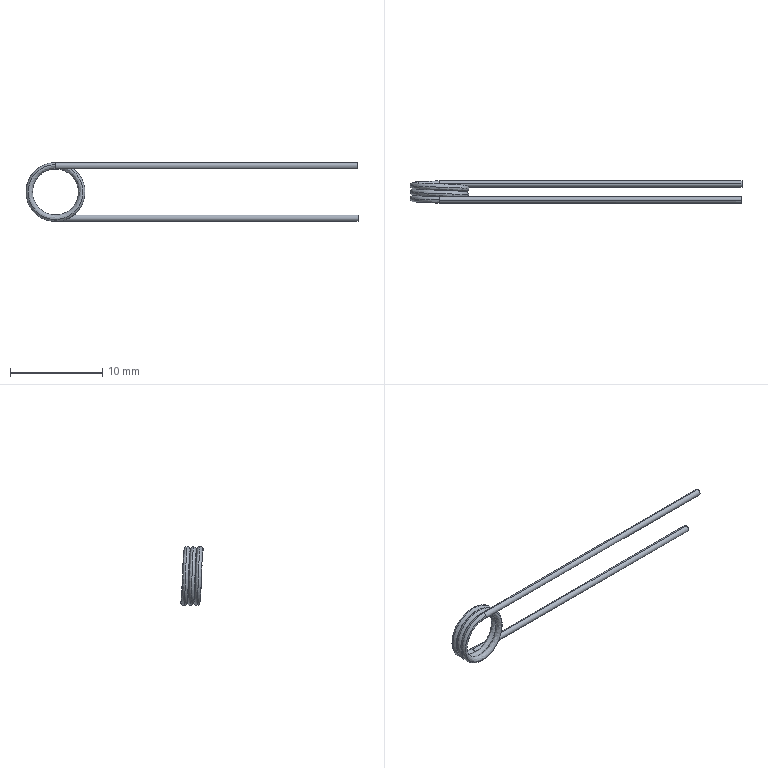Part | SolidWorks | features CompositeCurve 1, Helix 1, MoveFace 1, Sweep 1 | 1 solid | 9 faces | box 36.05 x 2.45 x 6.4 mm | volume 41.978 mm3 | cylinder 4 | spline 3 | plane 2 | commonest cylinder face diameters 0.7 x4
STEP:
#1=CARTESIAN_POINT('',(32.85,1.75,-3.2));
#2=VERTEX_POINT('',#1);
#3=CARTESIAN_POINT('',(32.85,1.75,-2.5));
#4=VERTEX_POINT('',#3);
#5=CARTESIAN_POINT('',(32.85,1.75,-2.85));
#6=DIRECTION('',(1.,0.,0.));
#7=DIRECTION('',(0.,0.00009155,-1.));
#8=AXIS2_PLACEMENT_3D('',#5,#6,#7);
#9=CIRCLE('',#8,0.35);
#10=EDGE_CURVE('',#2,#4,#9,.T.);
#11=ORIENTED_EDGE('',*,*,#10,.F.);
#12=CARTESIAN_POINT('',(-0.000000536,1.75,-3.2));
#13=VERTEX_POINT('',#12);
#14=CARTESIAN_POINT('',(12.85,1.75,-3.2));
#15=DIRECTION('',(-1.,0.,0.));
#16=VECTOR('',#15,1000.);
#17=LINE('',#14,#16);
#18=EDGE_CURVE('',#2,#13,#17,.T.);
#19=ORIENTED_EDGE('',*,*,#18,.T.);
#20=CARTESIAN_POINT('',(-0.006305,2.074,-2.979));
#21=VERTEX_POINT('',#20);
#22=CARTESIAN_POINT('',(0.,1.75,-2.85));
#23=DIRECTION('',(1.,0.,0.));
#24=DIRECTION('',(0.,0.00009155,-1.));
#25=AXIS2_PLACEMENT_3D('',#22,#23,#24);
#26=CIRCLE('',#25,0.35);
#27=EDGE_CURVE('',#13,#21,#26,.T.);
#28=ORIENTED_EDGE('',*,*,#27,.T.);
#29=CARTESIAN_POINT('',(0.,1.75,-2.5));
#30=VERTEX_POINT('',#29);
#31=CARTESIAN_POINT('',(0.,1.75,-2.85));
#32=DIRECTION('',(1.,0.,0.));
#33=DIRECTION('',(0.,0.00009155,-1.));
#34=AXIS2_PLACEMENT_3D('',#31,#32,#33);
#35=CIRCLE('',#34,0.35);
#36=EDGE_CURVE('',#21,#30,#35,.T.);
#37=ORIENTED_EDGE('',*,*,#36,.T.);
#38=CARTESIAN_POINT('',(12.85,1.75,-2.5));
#39=DIRECTION('',(-1.,0.,0.));
#40=VECTOR('',#39,1000.);
#41=LINE('',#38,#40);
#42=EDGE_CURVE('',#4,#30,#41,.T.);
#43=ORIENTED_EDGE('',*,*,#42,.F.);
#44=EDGE_LOOP('',(#11,#19,#28,#37,#43));
#45=FACE_OUTER_BOUND('',#44,.T.);
#46=CARTESIAN_POINT('',(12.85,1.75,-2.85));
#47=DIRECTION('',(-1.,0.,0.));
#48=DIRECTION('',(0.,0.,1.));
#49=AXIS2_PLACEMENT_3D('',#46,#47,#48);
#50=CYLINDRICAL_SURFACE('',#49,0.35);
#51=ADVANCED_FACE('',(#45),#50,.T.);
#52=CARTESIAN_POINT('',(0.006305,0.3239,2.979));
#53=VERTEX_POINT('',#52);
#54=CARTESIAN_POINT('',(0.,0.,3.2));
#55=VERTEX_POINT('',#54);
#56=CARTESIAN_POINT('',(0.006305,0.3239,2.979));
#57=CARTESIAN_POINT('',(0.01048,0.2681,3.104));
#58=CARTESIAN_POINT('',(0.005425,0.1388,3.2));
#59=CARTESIAN_POINT('',(0.,0.,3.2));
#60=B_SPLINE_CURVE_WITH_KNOTS('',3,(#56,#57,#58,#59),.UNSPECIFIED.,.F.,.F.,(4,4),(0.00002721,0.1895),.UNSPECIFIED.);
#61=EDGE_CURVE('',#53,#55,#60,.T.);
#62=ORIENTED_EDGE('',*,*,#61,.T.);
#63=CARTESIAN_POINT('',(32.85,0.,3.2));
#64=VERTEX_POINT('',#63);
#65=CARTESIAN_POINT('',(0.,0.,3.2));
#66=DIRECTION('',(1.,0.,0.));
#67=VECTOR('',#66,1000.);
#68=LINE('',#65,#67);
#69=EDGE_CURVE('',#55,#64,#68,.T.);
#70=ORIENTED_EDGE('',*,*,#69,.T.);
#71=CARTESIAN_POINT('',(32.85,0.,2.5));
#72=VERTEX_POINT('',#71);
#73=CARTESIAN_POINT('',(32.85,0.,2.85));
#74=DIRECTION('',(-1.,0.,0.));
#75=DIRECTION('',(0.,0.,1.));
#76=AXIS2_PLACEMENT_3D('',#73,#74,#75);
#77=CIRCLE('',#76,0.35);
#78=EDGE_CURVE('',#64,#72,#77,.T.);
#79=ORIENTED_EDGE('',*,*,#78,.T.);
#80=CARTESIAN_POINT('',(0.,0.,2.5));
#81=VERTEX_POINT('',#80);
#82=CARTESIAN_POINT('',(0.,0.,2.5));
#83=DIRECTION('',(1.,0.,0.));
#84=VECTOR('',#83,1000.);
#85=LINE('',#82,#84);
#86=EDGE_CURVE('',#81,#72,#85,.T.);
#87=ORIENTED_EDGE('',*,*,#86,.F.);
#88=CARTESIAN_POINT('',(0.,0.,2.85));
#89=DIRECTION('',(-1.,0.,0.));
#90=DIRECTION('',(0.,0.,1.));
#91=AXIS2_PLACEMENT_3D('',#88,#89,#90);
#92=CIRCLE('',#91,0.35);
#93=EDGE_CURVE('',#53,#81,#92,.T.);
#94=ORIENTED_EDGE('',*,*,#93,.F.);
#95=EDGE_LOOP('',(#62,#70,#79,#87,#94));
#96=FACE_OUTER_BOUND('',#95,.T.);
#97=CARTESIAN_POINT('',(0.,0.,2.85));
#98=DIRECTION('',(1.,0.,0.));
#99=DIRECTION('',(0.,0.,-1.));
#100=AXIS2_PLACEMENT_3D('',#97,#98,#99);
#101=CYLINDRICAL_SURFACE('',#100,0.35);
#102=ADVANCED_FACE('',(#96),#101,.T.);
#103=ORIENTED_EDGE('',*,*,#18,.F.);
#104=CARTESIAN_POINT('',(32.85,1.75,-2.85));
#105=DIRECTION('',(1.,0.,0.));
#106=DIRECTION('',(0.,0.00009155,-1.));
#107=AXIS2_PLACEMENT_3D('',#104,#105,#106);
#108=CIRCLE('',#107,0.35);
#109=EDGE_CURVE('',#4,#2,#108,.T.);
#110=ORIENTED_EDGE('',*,*,#109,.F.);
#111=ORIENTED_EDGE('',*,*,#42,.T.);
#112=CARTESIAN_POINT('',(0.006304,1.426,-2.979));
#113=VERTEX_POINT('',#112);
#114=CARTESIAN_POINT('',(0.,1.75,-2.85));
#115=DIRECTION('',(1.,0.,0.));
#116=DIRECTION('',(0.,0.00009155,-1.));
#117=AXIS2_PLACEMENT_3D('',#114,#115,#116);
#118=CIRCLE('',#117,0.35);
#119=EDGE_CURVE('',#30,#113,#118,.T.);
#120=ORIENTED_EDGE('',*,*,#119,.T.);
#121=CARTESIAN_POINT('',(0.,1.75,-2.85));
#122=DIRECTION('',(1.,0.,0.));
#123=DIRECTION('',(0.,0.00009155,-1.));
#124=AXIS2_PLACEMENT_3D('',#121,#122,#123);
#125=CIRCLE('',#124,0.35);
#126=EDGE_CURVE('',#113,#13,#125,.T.);
#127=ORIENTED_EDGE('',*,*,#126,.T.);
#128=EDGE_LOOP('',(#103,#110,#111,#120,#127));
#129=FACE_OUTER_BOUND('',#128,.T.);
#130=CARTESIAN_POINT('',(12.85,1.75,-2.85));
#131=DIRECTION('',(-1.,0.,0.));
#132=DIRECTION('',(0.,0.,1.));
#133=AXIS2_PLACEMENT_3D('',#130,#131,#132);
#134=CYLINDRICAL_SURFACE('',#133,0.35);
#135=ADVANCED_FACE('',(#129),#134,.T.);
#136=ORIENTED_EDGE('',*,*,#36,.F.);
#137=CARTESIAN_POINT('',(0.006305,0.3239,2.979));
#138=CARTESIAN_POINT('',(-0.7712,0.3519,2.981));
#139=CARTESIAN_POINT('',(-1.545,0.381,2.663));
#140=CARTESIAN_POINT('',(-2.649,0.4392,1.566));
#141=CARTESIAN_POINT('',(-2.975,0.4683,0.7939));
#142=CARTESIAN_POINT('',(-2.98,0.5195,-0.5733));
#143=CARTESIAN_POINT('',(-2.806,0.5413,-1.156));
#144=CARTESIAN_POINT('',(-2.162,0.585,-2.13));
#145=CARTESIAN_POINT('',(-1.69,0.6069,-2.521));
#146=CARTESIAN_POINT('',(-0.4324,0.658,-3.048));
#147=CARTESIAN_POINT('',(0.405,0.6871,-3.052));
#148=CARTESIAN_POINT('',(1.67,0.7383,-2.534));
#149=CARTESIAN_POINT('',(2.142,0.7601,-2.15));
#150=CARTESIAN_POINT('',(2.795,0.8037,-1.182));
#151=CARTESIAN_POINT('',(2.976,0.8257,-0.5972));
#152=CARTESIAN_POINT('',(2.981,0.8768,0.7668));
#153=CARTESIAN_POINT('',(2.665,0.9058,1.542));
#154=CARTESIAN_POINT('',(1.702,0.957,2.513));
#155=CARTESIAN_POINT('',(1.167,0.9788,2.801));
#156=CARTESIAN_POINT('',(0.02248,1.022,3.035));
#157=CARTESIAN_POINT('',(-0.587,1.044,2.978));
#158=CARTESIAN_POINT('',(-1.849,1.096,2.461));
#159=CARTESIAN_POINT('',(-2.445,1.125,1.872));
#160=CARTESIAN_POINT('',(-2.973,1.176,0.6109));
#161=CARTESIAN_POINT('',(-3.035,1.198,0.005944));
#162=CARTESIAN_POINT('',(-2.812,1.241,-1.14));
#163=CARTESIAN_POINT('',(-2.526,1.263,-1.682));
#164=CARTESIAN_POINT('',(-1.566,1.314,-2.65));
#165=CARTESIAN_POINT('',(-0.7938,1.343,-2.975));
#166=CARTESIAN_POINT('',(0.5733,1.395,-2.98));
#167=CARTESIAN_POINT('',(1.156,1.416,-2.806));
#168=CARTESIAN_POINT('',(2.13,1.46,-2.162));
#169=CARTESIAN_POINT('',(2.521,1.482,-1.69));
#170=CARTESIAN_POINT('',(3.048,1.533,-0.4324));
#171=CARTESIAN_POINT('',(3.052,1.562,0.405));
#172=CARTESIAN_POINT('',(2.534,1.613,1.67));
#173=CARTESIAN_POINT('',(2.15,1.635,2.142));
#174=CARTESIAN_POINT('',(1.182,1.679,2.795));
#175=CARTESIAN_POINT('',(0.5972,1.701,2.976));
#176=CARTESIAN_POINT('',(-0.7668,1.752,2.981));
#177=CARTESIAN_POINT('',(-1.542,1.781,2.665));
#178=CARTESIAN_POINT('',(-2.513,1.832,1.702));
#179=CARTESIAN_POINT('',(-2.801,1.854,1.167));
#180=CARTESIAN_POINT('',(-3.034,1.897,0.0225));
#181=CARTESIAN_POINT('',(-2.978,1.919,-0.587));
#182=CARTESIAN_POINT('',(-2.46,1.971,-1.85));
#183=CARTESIAN_POINT('',(-1.872,2.,-2.445));
#184=CARTESIAN_POINT('',(-0.7917,2.043,-2.897));
#185=CARTESIAN_POINT('',(-0.4042,2.058,-2.976));
#186=CARTESIAN_POINT('',(-0.006305,2.074,-2.979));
#187=B_SPLINE_CURVE_WITH_KNOTS('',3,(#137,#138,#139,#140,#141,#142,#143,#144,#145,#146,#147,#148,#149,#150,#151,#152,#153,#154,#155,#156,#157,#158,#159,#160,#161,#162,#163,#164,#165,#166,#167,#168,#169,#170,#171,#172,#173,#174,#175,#176,#177,#178,#179,#180,#181,#182,#183,#184,#185,#186),.UNSPECIFIED.,.F.,.F.,(4,2,2,2,2,2,2,2,2,2,2,2,2,2,2,2,2,2,2,2,2,2,2,2,4),(0.,0.04998,0.09999,0.1375,0.175,0.225,0.2625,0.3,0.35,0.3875,0.425,0.475,0.5125,0.55,0.6,0.6375,0.675,0.725,0.7625,0.8,0.85,0.8875,0.925,0.975,1.),.UNSPECIFIED.);
#188=EDGE_CURVE('',#53,#21,#187,.T.);
#189=ORIENTED_EDGE('',*,*,#188,.F.);
#190=ORIENTED_EDGE('',*,*,#93,.T.);
#191=CARTESIAN_POINT('',(-0.006304,-0.3239,2.979));
#192=VERTEX_POINT('',#191);
#193=CARTESIAN_POINT('',(0.,0.,2.85));
#194=DIRECTION('',(-1.,0.,0.));
#195=DIRECTION('',(0.,0.,1.));
#196=AXIS2_PLACEMENT_3D('',#193,#194,#195);
#197=CIRCLE('',#196,0.35);
#198=EDGE_CURVE('',#81,#192,#197,.T.);
#199=ORIENTED_EDGE('',*,*,#198,.T.);
#200=CARTESIAN_POINT('',(0.006304,1.426,-2.979));
#201=CARTESIAN_POINT('',(-0.379,1.413,-2.98));
#202=CARTESIAN_POINT('',(-0.7673,1.398,-2.904));
#203=CARTESIAN_POINT('',(-1.851,1.354,-2.461));
#204=CARTESIAN_POINT('',(-2.445,1.325,-1.871));
#205=CARTESIAN_POINT('',(-2.973,1.274,-0.6122));
#206=CARTESIAN_POINT('',(-3.035,1.252,-0.003211));
#207=CARTESIAN_POINT('',(-2.811,1.209,1.143));
#208=CARTESIAN_POINT('',(-2.527,1.187,1.681));
#209=CARTESIAN_POINT('',(-1.565,1.136,2.652));
#210=CARTESIAN_POINT('',(-0.792,1.107,2.975));
#211=CARTESIAN_POINT('',(0.572,1.056,2.981));
#212=CARTESIAN_POINT('',(1.158,1.034,2.805));
#213=CARTESIAN_POINT('',(2.132,0.99,2.16));
#214=CARTESIAN_POINT('',(2.52,0.9682,1.692));
#215=CARTESIAN_POINT('',(3.049,0.917,0.4308));
#216=CARTESIAN_POINT('',(3.052,0.8879,-0.4067));
#217=CARTESIAN_POINT('',(2.535,0.8368,-1.669));
#218=CARTESIAN_POINT('',(2.148,0.8149,-2.144));
#219=CARTESIAN_POINT('',(1.18,0.7712,-2.796));
#220=CARTESIAN_POINT('',(0.5985,0.7494,-2.976));
#221=CARTESIAN_POINT('',(-0.7686,0.6982,-2.981));
#222=CARTESIAN_POINT('',(-1.544,0.6692,-2.664));
#223=CARTESIAN_POINT('',(-2.512,0.6181,-1.703));
#224=CARTESIAN_POINT('',(-2.802,0.5961,-1.164));
#225=CARTESIAN_POINT('',(-3.035,0.5525,-0.01977));
#226=CARTESIAN_POINT('',(-2.978,0.5307,0.5858));
#227=CARTESIAN_POINT('',(-2.46,0.4795,1.851));
#228=CARTESIAN_POINT('',(-1.87,0.4504,2.445));
#229=CARTESIAN_POINT('',(-0.6122,0.3993,2.973));
#230=CARTESIAN_POINT('',(-0.003226,0.3774,3.035));
#231=CARTESIAN_POINT('',(1.143,0.3337,2.811));
#232=CARTESIAN_POINT('',(1.681,0.3119,2.527));
#233=CARTESIAN_POINT('',(2.652,0.2607,1.565));
#234=CARTESIAN_POINT('',(2.975,0.2317,0.792));
#235=CARTESIAN_POINT('',(2.981,0.1806,-0.572));
#236=CARTESIAN_POINT('',(2.805,0.1586,-1.158));
#237=CARTESIAN_POINT('',(2.16,0.115,-2.132));
#238=CARTESIAN_POINT('',(1.692,0.09317,-2.52));
#239=CARTESIAN_POINT('',(0.4308,0.04196,-3.049));
#240=CARTESIAN_POINT('',(-0.4067,0.01292,-3.052));
#241=CARTESIAN_POINT('',(-1.669,-0.03818,-2.535));
#242=CARTESIAN_POINT('',(-2.144,-0.06013,-2.148));
#243=CARTESIAN_POINT('',(-2.796,-0.1038,-1.18));
#244=CARTESIAN_POINT('',(-2.976,-0.1256,-0.5985));
#245=CARTESIAN_POINT('',(-2.981,-0.1768,0.7687));
#246=CARTESIAN_POINT('',(-2.663,-0.2059,1.544));
#247=CARTESIAN_POINT('',(-1.567,-0.2642,2.65));
#248=CARTESIAN_POINT('',(-0.7966,-0.2932,2.975));
#249=CARTESIAN_POINT('',(-0.006304,-0.3239,2.979));
#250=B_SPLINE_CURVE_WITH_KNOTS('',3,(#200,#201,#202,#203,#204,#205,#206,#207,#208,#209,#210,#211,#212,#213,#214,#215,#216,#217,#218,#219,#220,#221,#222,#223,#224,#225,#226,#227,#228,#229,#230,#231,#232,#233,#234,#235,#236,#237,#238,#239,#240,#241,#242,#243,#244,#245,#246,#247,#248,#249),.UNSPECIFIED.,.F.,.F.,(4,2,2,2,2,2,2,2,2,2,2,2,2,2,2,2,2,2,2,2,2,2,2,2,4),(0.,0.02496,0.07501,0.1125,0.15,0.2,0.2375,0.275,0.325,0.3625,0.4,0.45,0.4875,0.525,0.575,0.6125,0.65,0.7,0.7375,0.775,0.825,0.8625,0.9,0.95,1.),.UNSPECIFIED.);
#251=EDGE_CURVE('',#113,#192,#250,.T.);
#252=ORIENTED_EDGE('',*,*,#251,.F.);
#253=ORIENTED_EDGE('',*,*,#119,.F.);
#254=EDGE_LOOP('',(#136,#189,#190,#199,#252,#253));
#255=FACE_OUTER_BOUND('',#254,.T.);
#256=CARTESIAN_POINT('',(-0.01261,2.073,-2.978));
#257=CARTESIAN_POINT('',(-0.9931,2.036,-2.974));
#258=CARTESIAN_POINT('',(-1.942,2.,-2.452));
#259=CARTESIAN_POINT('',(-3.022,1.927,-0.8338));
#260=CARTESIAN_POINT('',(-3.123,1.89,0.2539));
#261=CARTESIAN_POINT('',(-2.369,1.817,2.048));
#262=CARTESIAN_POINT('',(-1.523,1.781,2.732));
#263=CARTESIAN_POINT('',(0.3864,1.708,3.111));
#264=CARTESIAN_POINT('',(1.43,1.671,2.788));
#265=CARTESIAN_POINT('',(2.798,1.599,1.405));
#266=CARTESIAN_POINT('',(3.107,1.562,0.3615));
#267=CARTESIAN_POINT('',(2.726,1.489,-1.547));
#268=CARTESIAN_POINT('',(2.029,1.453,-2.388));
#269=CARTESIAN_POINT('',(0.2273,1.38,-3.123));
#270=CARTESIAN_POINT('',(-0.8551,1.343,-3.009));
#271=CARTESIAN_POINT('',(-2.473,1.271,-1.927));
#272=CARTESIAN_POINT('',(-2.982,1.234,-0.9604));
#273=CARTESIAN_POINT('',(-2.972,1.161,0.9852));
#274=CARTESIAN_POINT('',(-2.453,1.125,1.942));
#275=CARTESIAN_POINT('',(-0.8335,1.052,3.022));
#276=CARTESIAN_POINT('',(0.2539,1.015,3.123));
#277=CARTESIAN_POINT('',(2.048,0.9425,2.369));
#278=CARTESIAN_POINT('',(2.732,0.9059,1.523));
#279=CARTESIAN_POINT('',(3.111,0.8331,-0.3864));
#280=CARTESIAN_POINT('',(2.788,0.7965,-1.43));
#281=CARTESIAN_POINT('',(1.405,0.7237,-2.798));
#282=CARTESIAN_POINT('',(0.3615,0.6872,-3.107));
#283=CARTESIAN_POINT('',(-1.547,0.6143,-2.726));
#284=CARTESIAN_POINT('',(-2.388,0.5777,-2.029));
#285=CARTESIAN_POINT('',(-3.123,0.505,-0.2273));
#286=CARTESIAN_POINT('',(-3.009,0.4684,0.8554));
#287=CARTESIAN_POINT('',(-1.927,0.3956,2.473));
#288=CARTESIAN_POINT('',(-0.9676,0.3593,2.982));
#289=CARTESIAN_POINT('',(0.01261,0.3226,2.978));
#290=CARTESIAN_POINT('',(-0.0161,2.162,-2.771));
#291=CARTESIAN_POINT('',(-0.9269,2.125,-2.766));
#292=CARTESIAN_POINT('',(-1.811,2.089,-2.279));
#293=CARTESIAN_POINT('',(-2.813,2.016,-0.7712));
#294=CARTESIAN_POINT('',(-2.906,1.979,0.2409));
#295=CARTESIAN_POINT('',(-2.201,1.907,1.909));
#296=CARTESIAN_POINT('',(-1.413,1.87,2.545));
#297=CARTESIAN_POINT('',(0.3644,1.797,2.894));
#298=CARTESIAN_POINT('',(1.334,1.761,2.592));
#299=CARTESIAN_POINT('',(2.606,1.688,1.303));
#300=CARTESIAN_POINT('',(2.892,1.651,0.3318));
#301=CARTESIAN_POINT('',(2.535,1.579,-1.444));
#302=CARTESIAN_POINT('',(1.884,1.542,-2.225));
#303=CARTESIAN_POINT('',(0.2064,1.469,-2.907));
#304=CARTESIAN_POINT('',(-0.8001,1.433,-2.799));
#305=CARTESIAN_POINT('',(-2.304,1.36,-1.789));
#306=CARTESIAN_POINT('',(-2.777,1.323,-0.8894));
#307=CARTESIAN_POINT('',(-2.764,1.25,0.9216));
#308=CARTESIAN_POINT('',(-2.279,1.214,1.81));
#309=CARTESIAN_POINT('',(-0.771,1.141,2.814));
#310=CARTESIAN_POINT('',(0.2409,1.104,2.906));
#311=CARTESIAN_POINT('',(1.909,1.032,2.201));
#312=CARTESIAN_POINT('',(2.545,0.9951,1.413));
#313=CARTESIAN_POINT('',(2.894,0.9223,-0.3644));
#314=CARTESIAN_POINT('',(2.592,0.8857,-1.334));
#315=CARTESIAN_POINT('',(1.303,0.8129,-2.606));
#316=CARTESIAN_POINT('',(0.3318,0.7764,-2.892));
#317=CARTESIAN_POINT('',(-1.444,0.7035,-2.535));
#318=CARTESIAN_POINT('',(-2.225,0.667,-1.884));
#319=CARTESIAN_POINT('',(-2.907,0.5942,-0.2064));
#320=CARTESIAN_POINT('',(-2.798,0.5576,0.8003));
#321=CARTESIAN_POINT('',(-1.789,0.4848,2.304));
#322=CARTESIAN_POINT('',(-0.8958,0.4485,2.776));
#323=CARTESIAN_POINT('',(0.0161,0.4118,2.771));
#324=CARTESIAN_POINT('',(-0.008888,1.977,-2.5));
#325=CARTESIAN_POINT('',(-0.8283,1.941,-2.497));
#326=CARTESIAN_POINT('',(-1.629,1.904,-2.059));
#327=CARTESIAN_POINT('',(-2.536,1.832,-0.7012));
#328=CARTESIAN_POINT('',(-2.622,1.795,0.2114));
#329=CARTESIAN_POINT('',(-1.989,1.722,1.718));
#330=CARTESIAN_POINT('',(-1.28,1.686,2.292));
#331=CARTESIAN_POINT('',(0.3232,1.613,2.612));
#332=CARTESIAN_POINT('',(1.199,1.576,2.341));
#333=CARTESIAN_POINT('',(2.349,1.503,1.18));
#334=CARTESIAN_POINT('',(2.608,1.467,0.3051));
#335=CARTESIAN_POINT('',(2.29,1.394,-1.298));
#336=CARTESIAN_POINT('',(1.704,1.358,-2.003));
#337=CARTESIAN_POINT('',(0.1914,1.285,-2.622));
#338=CARTESIAN_POINT('',(-0.716,1.248,-2.526));
#339=CARTESIAN_POINT('',(-2.075,1.175,-1.618));
#340=CARTESIAN_POINT('',(-2.503,1.139,-0.808));
#341=CARTESIAN_POINT('',(-2.495,1.066,0.8264));
#342=CARTESIAN_POINT('',(-2.06,1.029,1.628));
#343=CARTESIAN_POINT('',(-0.701,0.9565,2.537));
#344=CARTESIAN_POINT('',(0.2114,0.92,2.622));
#345=CARTESIAN_POINT('',(1.718,0.8471,1.989));
#346=CARTESIAN_POINT('',(2.292,0.8107,1.28));
#347=CARTESIAN_POINT('',(2.612,0.7378,-0.3232));
#348=CARTESIAN_POINT('',(2.341,0.7013,-1.199));
#349=CARTESIAN_POINT('',(1.18,0.6284,-2.349));
#350=CARTESIAN_POINT('',(0.3051,0.5919,-2.608));
#351=CARTESIAN_POINT('',(-1.298,0.519,-2.29));
#352=CARTESIAN_POINT('',(-2.003,0.4825,-1.704));
#353=CARTESIAN_POINT('',(-2.622,0.4096,-0.1914));
#354=CARTESIAN_POINT('',(-2.525,0.3732,0.7162));
#355=CARTESIAN_POINT('',(-1.619,0.3003,2.075));
#356=CARTESIAN_POINT('',(-0.8134,0.2639,2.503));
#357=CARTESIAN_POINT('',(0.008889,0.2274,2.5));
#358=CARTESIAN_POINT('',(0.008895,1.522,-2.5));
#359=CARTESIAN_POINT('',(-0.8105,1.486,-2.503));
#360=CARTESIAN_POINT('',(-1.614,1.45,-2.071));
#361=CARTESIAN_POINT('',(-2.532,1.377,-0.7193));
#362=CARTESIAN_POINT('',(-2.623,1.34,0.1927));
#363=CARTESIAN_POINT('',(-2.001,1.267,1.704));
#364=CARTESIAN_POINT('',(-1.296,1.231,2.283));
#365=CARTESIAN_POINT('',(0.3046,1.158,2.614));
#366=CARTESIAN_POINT('',(1.182,1.121,2.35));
#367=CARTESIAN_POINT('',(2.341,1.048,1.197));
#368=CARTESIAN_POINT('',(2.606,1.012,0.3236));
#369=CARTESIAN_POINT('',(2.299,0.9391,-1.282));
#370=CARTESIAN_POINT('',(1.719,0.9026,-1.991));
#371=CARTESIAN_POINT('',(0.2101,0.8297,-2.62));
#372=CARTESIAN_POINT('',(-0.6981,0.7933,-2.531));
#373=CARTESIAN_POINT('',(-2.064,0.7204,-1.633));
#374=CARTESIAN_POINT('',(-2.497,0.6839,-0.8259));
#375=CARTESIAN_POINT('',(-2.501,0.611,0.8087));
#376=CARTESIAN_POINT('',(-2.071,0.5745,1.614));
#377=CARTESIAN_POINT('',(-0.7191,0.5016,2.532));
#378=CARTESIAN_POINT('',(0.1927,0.4651,2.623));
#379=CARTESIAN_POINT('',(1.704,0.3922,2.001));
#380=CARTESIAN_POINT('',(2.283,0.3558,1.296));
#381=CARTESIAN_POINT('',(2.614,0.2829,-0.3046));
#382=CARTESIAN_POINT('',(2.35,0.2464,-1.182));
#383=CARTESIAN_POINT('',(1.197,0.1735,-2.341));
#384=CARTESIAN_POINT('',(0.3236,0.137,-2.606));
#385=CARTESIAN_POINT('',(-1.282,0.0641,-2.299));
#386=CARTESIAN_POINT('',(-1.991,0.02763,-1.719));
#387=CARTESIAN_POINT('',(-2.62,-0.04528,-0.2101));
#388=CARTESIAN_POINT('',(-2.531,-0.08173,0.6983));
#389=CARTESIAN_POINT('',(-1.633,-0.1546,2.064));
#390=CARTESIAN_POINT('',(-0.8313,-0.191,2.497));
#391=CARTESIAN_POINT('',(-0.008894,-0.2275,2.5));
#392=CARTESIAN_POINT('',(0.0161,1.338,-2.771));
#393=CARTESIAN_POINT('',(-0.8947,1.302,-2.777));
#394=CARTESIAN_POINT('',(-1.785,1.265,-2.3));
#395=CARTESIAN_POINT('',(-2.804,1.192,-0.804));
#396=CARTESIAN_POINT('',(-2.908,1.156,0.2071));
#397=CARTESIAN_POINT('',(-2.223,1.083,1.884));
#398=CARTESIAN_POINT('',(-1.443,1.046,2.528));
#399=CARTESIAN_POINT('',(0.3307,0.9736,2.899));
#400=CARTESIAN_POINT('',(1.304,0.937,2.608));
#401=CARTESIAN_POINT('',(2.591,0.8642,1.333));
#402=CARTESIAN_POINT('',(2.888,0.8277,0.3653));
#403=CARTESIAN_POINT('',(2.552,0.7548,-1.415));
#404=CARTESIAN_POINT('',(1.91,0.7183,-2.203));
#405=CARTESIAN_POINT('',(0.2402,0.6455,-2.904));
#406=CARTESIAN_POINT('',(-0.7677,0.6089,-2.808));
#407=CARTESIAN_POINT('',(-2.284,0.5361,-1.816));
#408=CARTESIAN_POINT('',(-2.766,0.4995,-0.9217));
#409=CARTESIAN_POINT('',(-2.775,0.4267,0.8895));
#410=CARTESIAN_POINT('',(-2.3,0.3902,1.784));
#411=CARTESIAN_POINT('',(-0.8038,0.3173,2.805));
#412=CARTESIAN_POINT('',(0.2071,0.2808,2.908));
#413=CARTESIAN_POINT('',(1.884,0.208,2.223));
#414=CARTESIAN_POINT('',(2.528,0.1714,1.443));
#415=CARTESIAN_POINT('',(2.899,0.09857,-0.3307));
#416=CARTESIAN_POINT('',(2.608,0.06204,-1.304));
#417=CARTESIAN_POINT('',(1.333,-0.01079,-2.591));
#418=CARTESIAN_POINT('',(0.3653,-0.0473,-2.888));
#419=CARTESIAN_POINT('',(-1.415,-0.1202,-2.552));
#420=CARTESIAN_POINT('',(-2.203,-0.1567,-1.91));
#421=CARTESIAN_POINT('',(-2.904,-0.2295,-0.2402));
#422=CARTESIAN_POINT('',(-2.807,-0.2661,0.7679));
#423=CARTESIAN_POINT('',(-1.816,-0.3389,2.283));
#424=CARTESIAN_POINT('',(-0.9282,-0.3752,2.766));
#425=CARTESIAN_POINT('',(-0.0161,-0.4119,2.771));
#426=CARTESIAN_POINT('',(0.01261,1.427,-2.978));
#427=CARTESIAN_POINT('',(-0.9679,1.391,-2.982));
#428=CARTESIAN_POINT('',(-1.922,1.354,-2.469));
#429=CARTESIAN_POINT('',(-3.015,1.282,-0.8595));
#430=CARTESIAN_POINT('',(-3.125,1.245,0.2275));
#431=CARTESIAN_POINT('',(-2.386,1.172,2.028));
#432=CARTESIAN_POINT('',(-1.546,1.136,2.72));
#433=CARTESIAN_POINT('',(0.36,1.063,3.114));
#434=CARTESIAN_POINT('',(1.406,1.026,2.8));
#435=CARTESIAN_POINT('',(2.787,0.9536,1.429));
#436=CARTESIAN_POINT('',(3.104,0.917,0.3878));
#437=CARTESIAN_POINT('',(2.739,0.8442,-1.524));
#438=CARTESIAN_POINT('',(2.049,0.8076,-2.37));
#439=CARTESIAN_POINT('',(0.2537,0.7349,-3.121));
#440=CARTESIAN_POINT('',(-0.8297,0.6983,-3.016));
#441=CARTESIAN_POINT('',(-2.457,0.6254,-1.948));
#442=CARTESIAN_POINT('',(-2.974,0.5889,-0.9857));
#443=CARTESIAN_POINT('',(-2.981,0.5161,0.96));
#444=CARTESIAN_POINT('',(-2.469,0.4795,1.921));
#445=CARTESIAN_POINT('',(-0.8592,0.4067,3.015));
#446=CARTESIAN_POINT('',(0.2275,0.3701,3.125));
#447=CARTESIAN_POINT('',(2.028,0.2974,2.386));
#448=CARTESIAN_POINT('',(2.72,0.2608,1.546));
#449=CARTESIAN_POINT('',(3.114,0.1879,-0.36));
#450=CARTESIAN_POINT('',(2.8,0.1514,-1.406));
#451=CARTESIAN_POINT('',(1.429,0.07861,-2.787));
#452=CARTESIAN_POINT('',(0.3878,0.04204,-3.104));
#453=CARTESIAN_POINT('',(-1.524,-0.03081,-2.739));
#454=CARTESIAN_POINT('',(-2.371,-0.06738,-2.049));
#455=CARTESIAN_POINT('',(-3.121,-0.1401,-0.2537));
#456=CARTESIAN_POINT('',(-3.016,-0.1767,0.83));
#457=CARTESIAN_POINT('',(-1.948,-0.2496,2.456));
#458=CARTESIAN_POINT('',(-0.993,-0.2858,2.974));
#459=CARTESIAN_POINT('',(-0.01261,-0.3225,2.978));
#460=B_SPLINE_SURFACE_WITH_KNOTS('',3,3,((#256,#257,#258,#259,#260,#261,#262,#263,#264,#265,#266,#267,#268,#269,#270,#271,#272,#273,#274,#275,#276,#277,#278,#279,#280,#281,#282,#283,#284,#285,#286,#287,#288,#289),(#290,#291,#292,#293,#294,#295,#296,#297,#298,#299,#300,#301,#302,#303,#304,#305,#306,#307,#308,#309,#310,#311,#312,#313,#314,#315,#316,#317,#318,#319,#320,#321,#322,#323),(#324,#325,#326,#327,#328,#329,#330,#331,#332,#333,#334,#335,#336,#337,#338,#339,#340,#341,#342,#343,#344,#345,#346,#347,#348,#349,#350,#351,#352,#353,#354,#355,#356,#357),(#358,#359,#360,#361,#362,#363,#364,#365,#366,#367,#368,#369,#370,#371,#372,#373,#374,#375,#376,#377,#378,#379,#380,#381,#382,#383,#384,#385,#386,#387,#388,#389,#390,#391),(#392,#393,#394,#395,#396,#397,#398,#399,#400,#401,#402,#403,#404,#405,#406,#407,#408,#409,#410,#411,#412,#413,#414,#415,#416,#417,#418,#419,#420,#421,#422,#423,#424,#425),(#426,#427,#428,#429,#430,#431,#432,#433,#434,#435,#436,#437,#438,#439,#440,#441,#442,#443,#444,#445,#446,#447,#448,#449,#450,#451,#452,#453,#454,#455,#456,#457,#458,#459)),.UNSPECIFIED.,.F.,.F.,.F.,(4,2,4),(4,2,2,2,2,2,2,2,2,2,2,2,2,2,2,2,4),(0.1895,0.5,0.8106),(0.,0.0625,0.125,0.1875,0.25,0.3125,0.375,0.4375,0.5,0.5625,0.625,0.6875,0.75,0.8125,0.875,0.9375,1.),.UNSPECIFIED.);
#461=ADVANCED_FACE('',(#255),#460,.F.);
#462=ORIENTED_EDGE('',*,*,#126,.F.);
#463=ORIENTED_EDGE('',*,*,#251,.T.);
#464=CARTESIAN_POINT('',(0.,0.,3.2));
#465=CARTESIAN_POINT('',(-0.005423,-0.1387,3.2));
#466=CARTESIAN_POINT('',(-0.01048,-0.268,3.104));
#467=CARTESIAN_POINT('',(-0.006304,-0.3239,2.979));
#468=B_SPLINE_CURVE_WITH_KNOTS('',3,(#464,#465,#466,#467),.UNSPECIFIED.,.F.,.F.,(4,4),(0.8106,1.),.UNSPECIFIED.);
#469=EDGE_CURVE('',#55,#192,#468,.T.);
#470=ORIENTED_EDGE('',*,*,#469,.F.);
#471=CARTESIAN_POINT('',(-0.000000536,1.75,-3.2));
#472=CARTESIAN_POINT('',(-0.4215,1.735,-3.2));
#473=CARTESIAN_POINT('',(-0.8371,1.721,-3.117));
#474=CARTESIAN_POINT('',(-2.001,1.677,-2.635));
#475=CARTESIAN_POINT('',(-2.635,1.648,-2.));
#476=CARTESIAN_POINT('',(-3.197,1.597,-0.6438));
#477=CARTESIAN_POINT('',(-3.261,1.575,0.01064));
#478=CARTESIAN_POINT('',(-3.015,1.531,1.241));
#479=CARTESIAN_POINT('',(-2.708,1.51,1.817));
#480=CARTESIAN_POINT('',(-1.669,1.458,2.857));
#481=CARTESIAN_POINT('',(-0.8382,1.429,3.2));
#482=CARTESIAN_POINT('',(0.6287,1.378,3.2));
#483=CARTESIAN_POINT('',(1.258,1.356,3.008));
#484=CARTESIAN_POINT('',(2.3,1.313,2.311));
#485=CARTESIAN_POINT('',(2.715,1.291,1.807));
#486=CARTESIAN_POINT('',(3.278,1.239,0.4484));
#487=CARTESIAN_POINT('',(3.277,1.211,-0.4502));
#488=CARTESIAN_POINT('',(2.716,1.159,-1.805));
#489=CARTESIAN_POINT('',(2.298,1.137,-2.313));
#490=CARTESIAN_POINT('',(1.255,1.094,-3.01));
#491=CARTESIAN_POINT('',(0.6301,1.072,-3.2));
#492=CARTESIAN_POINT('',(-0.8402,1.021,-3.2));
#493=CARTESIAN_POINT('',(-1.67,0.9918,-2.855));
#494=CARTESIAN_POINT('',(-2.707,0.9406,-1.818));
#495=CARTESIAN_POINT('',(-3.017,0.9186,-1.238));
#496=CARTESIAN_POINT('',(-3.261,0.875,-0.007701));
#497=CARTESIAN_POINT('',(-3.198,0.8533,0.6424));
#498=CARTESIAN_POINT('',(-2.635,0.8019,2.001));
#499=CARTESIAN_POINT('',(-1.999,0.773,2.636));
#500=CARTESIAN_POINT('',(-0.6438,0.7218,3.197));
#501=CARTESIAN_POINT('',(0.01062,0.6999,3.261));
#502=CARTESIAN_POINT('',(1.241,0.6563,3.015));
#503=CARTESIAN_POINT('',(1.817,0.6345,2.708));
#504=CARTESIAN_POINT('',(2.857,0.5832,1.669));
#505=CARTESIAN_POINT('',(3.2,0.5543,0.8382));
#506=CARTESIAN_POINT('',(3.2,0.5031,-0.6287));
#507=CARTESIAN_POINT('',(3.008,0.4811,-1.258));
#508=CARTESIAN_POINT('',(2.311,0.4375,-2.3));
#509=CARTESIAN_POINT('',(1.807,0.4158,-2.715));
#510=CARTESIAN_POINT('',(0.4484,0.3644,-3.278));
#511=CARTESIAN_POINT('',(-0.4502,0.3355,-3.277));
#512=CARTESIAN_POINT('',(-1.805,0.2843,-2.716));
#513=CARTESIAN_POINT('',(-2.313,0.2624,-2.298));
#514=CARTESIAN_POINT('',(-3.01,0.2188,-1.255));
#515=CARTESIAN_POINT('',(-3.2,0.197,-0.6301));
#516=CARTESIAN_POINT('',(-3.2,0.1457,0.8403));
#517=CARTESIAN_POINT('',(-2.854,0.1167,1.671));
#518=CARTESIAN_POINT('',(-1.671,0.05831,2.854));
#519=CARTESIAN_POINT('',(-0.8425,0.02943,3.2));
#520=CARTESIAN_POINT('',(0.,0.,3.2));
#521=B_SPLINE_CURVE_WITH_KNOTS('',3,(#471,#472,#473,#474,#475,#476,#477,#478,#479,#480,#481,#482,#483,#484,#485,#486,#487,#488,#489,#490,#491,#492,#493,#494,#495,#496,#497,#498,#499,#500,#501,#502,#503,#504,#505,#506,#507,#508,#509,#510,#511,#512,#513,#514,#515,#516,#517,#518,#519,#520),.UNSPECIFIED.,.F.,.F.,(4,2,2,2,2,2,2,2,2,2,2,2,2,2,2,2,2,2,2,2,2,2,2,2,4),(0.,0.02496,0.07501,0.1125,0.15,0.2,0.2375,0.275,0.325,0.3625,0.4,0.45,0.4875,0.525,0.575,0.6125,0.65,0.7,0.7375,0.775,0.825,0.8625,0.9,0.95,1.),.UNSPECIFIED.);
#522=EDGE_CURVE('',#13,#55,#521,.T.);
#523=ORIENTED_EDGE('',*,*,#522,.F.);
#524=EDGE_LOOP('',(#462,#463,#470,#523));
#525=FACE_OUTER_BOUND('',#524,.T.);
#526=CARTESIAN_POINT('',(0.01261,1.427,-2.978));
#527=CARTESIAN_POINT('',(-0.379,1.413,-2.98));
#528=CARTESIAN_POINT('',(-0.7673,1.398,-2.904));
#529=CARTESIAN_POINT('',(-1.851,1.354,-2.461));
#530=CARTESIAN_POINT('',(-2.445,1.325,-1.871));
#531=CARTESIAN_POINT('',(-2.973,1.274,-0.6122));
#532=CARTESIAN_POINT('',(-3.035,1.252,-0.003211));
#533=CARTESIAN_POINT('',(-2.811,1.209,1.143));
#534=CARTESIAN_POINT('',(-2.527,1.187,1.681));
#535=CARTESIAN_POINT('',(-1.565,1.136,2.652));
#536=CARTESIAN_POINT('',(-0.792,1.107,2.975));
#537=CARTESIAN_POINT('',(0.572,1.056,2.981));
#538=CARTESIAN_POINT('',(1.158,1.034,2.805));
#539=CARTESIAN_POINT('',(2.132,0.99,2.16));
#540=CARTESIAN_POINT('',(2.52,0.9682,1.692));
#541=CARTESIAN_POINT('',(3.049,0.917,0.4308));
#542=CARTESIAN_POINT('',(3.052,0.8879,-0.4067));
#543=CARTESIAN_POINT('',(2.535,0.8368,-1.669));
#544=CARTESIAN_POINT('',(2.148,0.8149,-2.144));
#545=CARTESIAN_POINT('',(1.18,0.7712,-2.796));
#546=CARTESIAN_POINT('',(0.5985,0.7494,-2.976));
#547=CARTESIAN_POINT('',(-0.7686,0.6982,-2.981));
#548=CARTESIAN_POINT('',(-1.544,0.6692,-2.664));
#549=CARTESIAN_POINT('',(-2.512,0.6181,-1.703));
#550=CARTESIAN_POINT('',(-2.802,0.5961,-1.164));
#551=CARTESIAN_POINT('',(-3.035,0.5525,-0.01977));
#552=CARTESIAN_POINT('',(-2.978,0.5307,0.5858));
#553=CARTESIAN_POINT('',(-2.46,0.4795,1.851));
#554=CARTESIAN_POINT('',(-1.87,0.4504,2.445));
#555=CARTESIAN_POINT('',(-0.6122,0.3993,2.973));
#556=CARTESIAN_POINT('',(-0.003226,0.3774,3.035));
#557=CARTESIAN_POINT('',(1.143,0.3337,2.811));
#558=CARTESIAN_POINT('',(1.681,0.3119,2.527));
#559=CARTESIAN_POINT('',(2.652,0.2607,1.565));
#560=CARTESIAN_POINT('',(2.975,0.2317,0.792));
#561=CARTESIAN_POINT('',(2.981,0.1806,-0.572));
#562=CARTESIAN_POINT('',(2.805,0.1586,-1.158));
#563=CARTESIAN_POINT('',(2.16,0.115,-2.132));
#564=CARTESIAN_POINT('',(1.692,0.09317,-2.52));
#565=CARTESIAN_POINT('',(0.4308,0.04196,-3.049));
#566=CARTESIAN_POINT('',(-0.4067,0.01292,-3.052));
#567=CARTESIAN_POINT('',(-1.669,-0.03818,-2.535));
#568=CARTESIAN_POINT('',(-2.144,-0.06013,-2.148));
#569=CARTESIAN_POINT('',(-2.796,-0.1038,-1.18));
#570=CARTESIAN_POINT('',(-2.976,-0.1256,-0.5985));
#571=CARTESIAN_POINT('',(-2.981,-0.1768,0.7687));
#572=CARTESIAN_POINT('',(-2.663,-0.2059,1.544));
#573=CARTESIAN_POINT('',(-1.567,-0.2642,2.65));
#574=CARTESIAN_POINT('',(-0.7966,-0.2932,2.975));
#575=CARTESIAN_POINT('',(-0.01261,-0.3225,2.978));
#576=CARTESIAN_POINT('',(0.01048,1.482,-3.104));
#577=CARTESIAN_POINT('',(-0.3981,1.467,-3.106));
#578=CARTESIAN_POINT('',(-0.802,1.453,-3.026));
#579=CARTESIAN_POINT('',(-1.932,1.409,-2.563));
#580=CARTESIAN_POINT('',(-2.55,1.38,-1.948));
#581=CARTESIAN_POINT('',(-3.099,1.329,-0.6352));
#582=CARTESIAN_POINT('',(-3.163,1.307,-0.0004747));
#583=CARTESIAN_POINT('',(-2.929,1.263,1.194));
#584=CARTESIAN_POINT('',(-2.633,1.241,1.754));
#585=CARTESIAN_POINT('',(-1.628,1.19,2.766));
#586=CARTESIAN_POINT('',(-0.8233,1.161,3.102));
#587=CARTESIAN_POINT('',(0.5992,1.11,3.106));
#588=CARTESIAN_POINT('',(1.21,1.088,2.923));
#589=CARTESIAN_POINT('',(2.224,1.044,2.249));
#590=CARTESIAN_POINT('',(2.628,1.023,1.761));
#591=CARTESIAN_POINT('',(3.178,0.9714,0.4459));
#592=CARTESIAN_POINT('',(3.181,0.9425,-0.4263));
#593=CARTESIAN_POINT('',(2.641,0.8913,-1.742));
#594=CARTESIAN_POINT('',(2.237,0.8694,-2.236));
#595=CARTESIAN_POINT('',(1.227,0.8257,-2.915));
#596=CARTESIAN_POINT('',(0.6215,0.804,-3.102));
#597=CARTESIAN_POINT('',(-0.8043,0.7527,-3.107));
#598=CARTESIAN_POINT('',(-1.611,0.7237,-2.775));
#599=CARTESIAN_POINT('',(-2.62,0.6725,-1.773));
#600=CARTESIAN_POINT('',(-2.922,0.6506,-1.211));
#601=CARTESIAN_POINT('',(-3.163,0.607,-0.01804));
#602=CARTESIAN_POINT('',(-3.104,0.5852,0.613));
#603=CARTESIAN_POINT('',(-2.563,0.5339,1.932));
#604=CARTESIAN_POINT('',(-1.948,0.505,2.55));
#605=CARTESIAN_POINT('',(-0.6352,0.4538,3.099));
#606=CARTESIAN_POINT('',(-0.0004918,0.4319,3.163));
#607=CARTESIAN_POINT('',(1.194,0.3882,2.929));
#608=CARTESIAN_POINT('',(1.754,0.3665,2.633));
#609=CARTESIAN_POINT('',(2.766,0.3152,1.628));
#610=CARTESIAN_POINT('',(3.102,0.2862,0.8233));
#611=CARTESIAN_POINT('',(3.106,0.235,-0.5992));
#612=CARTESIAN_POINT('',(2.923,0.2131,-1.21));
#613=CARTESIAN_POINT('',(2.249,0.1695,-2.224));
#614=CARTESIAN_POINT('',(1.761,0.1477,-2.628));
#615=CARTESIAN_POINT('',(0.4459,0.09641,-3.178));
#616=CARTESIAN_POINT('',(-0.4263,0.06746,-3.181));
#617=CARTESIAN_POINT('',(-1.742,0.01629,-2.641));
#618=CARTESIAN_POINT('',(-2.236,-0.005646,-2.237));
#619=CARTESIAN_POINT('',(-2.915,-0.04927,-1.227));
#620=CARTESIAN_POINT('',(-3.102,-0.07105,-0.6215));
#621=CARTESIAN_POINT('',(-3.107,-0.1223,0.8044));
#622=CARTESIAN_POINT('',(-2.774,-0.1514,1.612));
#623=CARTESIAN_POINT('',(-1.631,-0.2097,2.763));
#624=CARTESIAN_POINT('',(-0.8278,-0.2386,3.102));
#625=CARTESIAN_POINT('',(-0.01048,-0.268,3.104));
#626=CARTESIAN_POINT('',(0.005423,1.611,-3.2));
#627=CARTESIAN_POINT('',(-0.416,1.597,-3.201));
#628=CARTESIAN_POINT('',(-0.8318,1.582,-3.118));
#629=CARTESIAN_POINT('',(-1.996,1.538,-2.639));
#630=CARTESIAN_POINT('',(-2.632,1.509,-2.004));
#631=CARTESIAN_POINT('',(-3.196,1.458,-0.6492));
#632=CARTESIAN_POINT('',(-3.261,1.436,0.005106));
#633=CARTESIAN_POINT('',(-3.018,1.393,1.236));
#634=CARTESIAN_POINT('',(-2.711,1.371,1.813));
#635=CARTESIAN_POINT('',(-1.673,1.319,2.854));
#636=CARTESIAN_POINT('',(-0.8436,1.291,3.199));
#637=CARTESIAN_POINT('',(0.6232,1.239,3.201));
#638=CARTESIAN_POINT('',(1.253,1.217,3.011));
#639=CARTESIAN_POINT('',(2.296,1.174,2.315));
#640=CARTESIAN_POINT('',(2.712,1.152,1.811));
#641=CARTESIAN_POINT('',(3.277,1.101,0.4539));
#642=CARTESIAN_POINT('',(3.278,1.072,-0.4446));
#643=CARTESIAN_POINT('',(2.719,1.021,-1.801));
#644=CARTESIAN_POINT('',(2.302,0.9986,-2.309));
#645=CARTESIAN_POINT('',(1.26,0.955,-3.007));
#646=CARTESIAN_POINT('',(0.6356,0.9333,-3.199));
#647=CARTESIAN_POINT('',(-0.8348,0.8819,-3.201));
#648=CARTESIAN_POINT('',(-1.665,0.853,-2.858));
#649=CARTESIAN_POINT('',(-2.704,0.8018,-1.823));
#650=CARTESIAN_POINT('',(-3.014,0.7799,-1.243));
#651=CARTESIAN_POINT('',(-3.261,0.7363,-0.01323));
#652=CARTESIAN_POINT('',(-3.199,0.7145,0.637));
#653=CARTESIAN_POINT('',(-2.638,0.6632,1.996));
#654=CARTESIAN_POINT('',(-2.003,0.6343,2.632));
#655=CARTESIAN_POINT('',(-0.6492,0.583,3.196));
#656=CARTESIAN_POINT('',(0.005088,0.5611,3.261));
#657=CARTESIAN_POINT('',(1.236,0.5175,3.018));
#658=CARTESIAN_POINT('',(1.813,0.4958,2.711));
#659=CARTESIAN_POINT('',(2.854,0.4444,1.673));
#660=CARTESIAN_POINT('',(3.199,0.4155,0.8437));
#661=CARTESIAN_POINT('',(3.201,0.3643,-0.6232));
#662=CARTESIAN_POINT('',(3.011,0.3424,-1.253));
#663=CARTESIAN_POINT('',(2.315,0.2988,-2.296));
#664=CARTESIAN_POINT('',(1.811,0.277,-2.712));
#665=CARTESIAN_POINT('',(0.4539,0.2257,-3.277));
#666=CARTESIAN_POINT('',(-0.4446,0.1968,-3.278));
#667=CARTESIAN_POINT('',(-1.801,0.1455,-2.719));
#668=CARTESIAN_POINT('',(-2.309,0.1236,-2.302));
#669=CARTESIAN_POINT('',(-3.007,0.08004,-1.26));
#670=CARTESIAN_POINT('',(-3.199,0.05826,-0.6356));
#671=CARTESIAN_POINT('',(-3.201,0.006904,0.8348));
#672=CARTESIAN_POINT('',(-2.857,-0.02205,1.666));
#673=CARTESIAN_POINT('',(-1.676,-0.08045,2.852));
#674=CARTESIAN_POINT('',(-0.848,-0.1093,3.199));
#675=CARTESIAN_POINT('',(-0.005424,-0.1388,3.2));
#676=CARTESIAN_POINT('',(-0.000001252,1.75,-3.2));
#677=CARTESIAN_POINT('',(-0.4215,1.735,-3.2));
#678=CARTESIAN_POINT('',(-0.8371,1.721,-3.117));
#679=CARTESIAN_POINT('',(-2.001,1.677,-2.635));
#680=CARTESIAN_POINT('',(-2.635,1.648,-2.));
#681=CARTESIAN_POINT('',(-3.197,1.597,-0.6438));
#682=CARTESIAN_POINT('',(-3.261,1.575,0.01064));
#683=CARTESIAN_POINT('',(-3.015,1.531,1.241));
#684=CARTESIAN_POINT('',(-2.708,1.51,1.817));
#685=CARTESIAN_POINT('',(-1.669,1.458,2.857));
#686=CARTESIAN_POINT('',(-0.8382,1.429,3.2));
#687=CARTESIAN_POINT('',(0.6287,1.378,3.2));
#688=CARTESIAN_POINT('',(1.258,1.356,3.008));
#689=CARTESIAN_POINT('',(2.3,1.313,2.311));
#690=CARTESIAN_POINT('',(2.715,1.291,1.807));
#691=CARTESIAN_POINT('',(3.278,1.239,0.4484));
#692=CARTESIAN_POINT('',(3.277,1.211,-0.4502));
#693=CARTESIAN_POINT('',(2.716,1.159,-1.805));
#694=CARTESIAN_POINT('',(2.298,1.137,-2.313));
#695=CARTESIAN_POINT('',(1.255,1.094,-3.01));
#696=CARTESIAN_POINT('',(0.6301,1.072,-3.2));
#697=CARTESIAN_POINT('',(-0.8402,1.021,-3.2));
#698=CARTESIAN_POINT('',(-1.67,0.9918,-2.855));
#699=CARTESIAN_POINT('',(-2.707,0.9406,-1.818));
#700=CARTESIAN_POINT('',(-3.017,0.9186,-1.238));
#701=CARTESIAN_POINT('',(-3.261,0.875,-0.007701));
#702=CARTESIAN_POINT('',(-3.198,0.8533,0.6424));
#703=CARTESIAN_POINT('',(-2.635,0.8019,2.001));
#704=CARTESIAN_POINT('',(-1.999,0.773,2.636));
#705=CARTESIAN_POINT('',(-0.6438,0.7218,3.197));
#706=CARTESIAN_POINT('',(0.01062,0.6999,3.261));
#707=CARTESIAN_POINT('',(1.241,0.6563,3.015));
#708=CARTESIAN_POINT('',(1.817,0.6345,2.708));
#709=CARTESIAN_POINT('',(2.857,0.5832,1.669));
#710=CARTESIAN_POINT('',(3.2,0.5543,0.8382));
#711=CARTESIAN_POINT('',(3.2,0.5031,-0.6287));
#712=CARTESIAN_POINT('',(3.008,0.4811,-1.258));
#713=CARTESIAN_POINT('',(2.311,0.4375,-2.3));
#714=CARTESIAN_POINT('',(1.807,0.4158,-2.715));
#715=CARTESIAN_POINT('',(0.4484,0.3644,-3.278));
#716=CARTESIAN_POINT('',(-0.4502,0.3355,-3.277));
#717=CARTESIAN_POINT('',(-1.805,0.2843,-2.716));
#718=CARTESIAN_POINT('',(-2.313,0.2624,-2.298));
#719=CARTESIAN_POINT('',(-3.01,0.2188,-1.255));
#720=CARTESIAN_POINT('',(-3.2,0.197,-0.6301));
#721=CARTESIAN_POINT('',(-3.2,0.1457,0.8403));
#722=CARTESIAN_POINT('',(-2.854,0.1167,1.671));
#723=CARTESIAN_POINT('',(-1.671,0.05831,2.854));
#724=CARTESIAN_POINT('',(-0.8425,0.02943,3.2));
#725=CARTESIAN_POINT('',(0.,0.,3.2));
#726=B_SPLINE_SURFACE_WITH_KNOTS('',3,3,((#526,#527,#528,#529,#530,#531,#532,#533,#534,#535,#536,#537,#538,#539,#540,#541,#542,#543,#544,#545,#546,#547,#548,#549,#550,#551,#552,#553,#554,#555,#556,#557,#558,#559,#560,#561,#562,#563,#564,#565,#566,#567,#568,#569,#570,#571,#572,#573,#574,#575),(#576,#577,#578,#579,#580,#581,#582,#583,#584,#585,#586,#587,#588,#589,#590,#591,#592,#593,#594,#595,#596,#597,#598,#599,#600,#601,#602,#603,#604,#605,#606,#607,#608,#609,#610,#611,#612,#613,#614,#615,#616,#617,#618,#619,#620,#621,#622,#623,#624,#625),(#626,#627,#628,#629,#630,#631,#632,#633,#634,#635,#636,#637,#638,#639,#640,#641,#642,#643,#644,#645,#646,#647,#648,#649,#650,#651,#652,#653,#654,#655,#656,#657,#658,#659,#660,#661,#662,#663,#664,#665,#666,#667,#668,#669,#670,#671,#672,#673,#674,#675),(#676,#677,#678,#679,#680,#681,#682,#683,#684,#685,#686,#687,#688,#689,#690,#691,#692,#693,#694,#695,#696,#697,#698,#699,#700,#701,#702,#703,#704,#705,#706,#707,#708,#709,#710,#711,#712,#713,#714,#715,#716,#717,#718,#719,#720,#721,#722,#723,#724,#725)),.UNSPECIFIED.,.F.,.F.,.F.,(4,4),(4,2,2,2,2,2,2,2,2,2,2,2,2,2,2,2,2,2,2,2,2,2,2,2,4),(0.8106,1.),(0.,0.02496,0.07501,0.1125,0.15,0.2,0.2375,0.275,0.325,0.3625,0.4,0.45,0.4875,0.525,0.575,0.6125,0.65,0.7,0.7375,0.775,0.825,0.8625,0.9,0.95,1.),.UNSPECIFIED.);
#727=ADVANCED_FACE('',(#525),#726,.F.);
#728=ORIENTED_EDGE('',*,*,#27,.F.);
#729=ORIENTED_EDGE('',*,*,#522,.T.);
#730=ORIENTED_EDGE('',*,*,#61,.F.);
#731=ORIENTED_EDGE('',*,*,#188,.T.);
#732=EDGE_LOOP('',(#728,#729,#730,#731));
#733=FACE_OUTER_BOUND('',#732,.T.);
#734=CARTESIAN_POINT('',(-0.000001252,1.75,-3.2));
#735=CARTESIAN_POINT('',(-0.4215,1.735,-3.2));
#736=CARTESIAN_POINT('',(-0.8371,1.721,-3.117));
#737=CARTESIAN_POINT('',(-2.001,1.677,-2.635));
#738=CARTESIAN_POINT('',(-2.635,1.648,-2.));
#739=CARTESIAN_POINT('',(-3.197,1.597,-0.6438));
#740=CARTESIAN_POINT('',(-3.261,1.575,0.01064));
#741=CARTESIAN_POINT('',(-3.015,1.531,1.241));
#742=CARTESIAN_POINT('',(-2.708,1.51,1.817));
#743=CARTESIAN_POINT('',(-1.669,1.458,2.857));
#744=CARTESIAN_POINT('',(-0.8382,1.429,3.2));
#745=CARTESIAN_POINT('',(0.6287,1.378,3.2));
#746=CARTESIAN_POINT('',(1.258,1.356,3.008));
#747=CARTESIAN_POINT('',(2.3,1.313,2.311));
#748=CARTESIAN_POINT('',(2.715,1.291,1.807));
#749=CARTESIAN_POINT('',(3.278,1.239,0.4484));
#750=CARTESIAN_POINT('',(3.277,1.211,-0.4502));
#751=CARTESIAN_POINT('',(2.716,1.159,-1.805));
#752=CARTESIAN_POINT('',(2.298,1.137,-2.313));
#753=CARTESIAN_POINT('',(1.255,1.094,-3.01));
#754=CARTESIAN_POINT('',(0.6301,1.072,-3.2));
#755=CARTESIAN_POINT('',(-0.8402,1.021,-3.2));
#756=CARTESIAN_POINT('',(-1.67,0.9918,-2.855));
#757=CARTESIAN_POINT('',(-2.707,0.9406,-1.818));
#758=CARTESIAN_POINT('',(-3.017,0.9186,-1.238));
#759=CARTESIAN_POINT('',(-3.261,0.875,-0.007701));
#760=CARTESIAN_POINT('',(-3.198,0.8533,0.6424));
#761=CARTESIAN_POINT('',(-2.635,0.8019,2.001));
#762=CARTESIAN_POINT('',(-1.999,0.773,2.636));
#763=CARTESIAN_POINT('',(-0.6438,0.7218,3.197));
#764=CARTESIAN_POINT('',(0.01062,0.6999,3.261));
#765=CARTESIAN_POINT('',(1.241,0.6563,3.015));
#766=CARTESIAN_POINT('',(1.817,0.6345,2.708));
#767=CARTESIAN_POINT('',(2.857,0.5832,1.669));
#768=CARTESIAN_POINT('',(3.2,0.5543,0.8382));
#769=CARTESIAN_POINT('',(3.2,0.5031,-0.6287));
#770=CARTESIAN_POINT('',(3.008,0.4811,-1.258));
#771=CARTESIAN_POINT('',(2.311,0.4375,-2.3));
#772=CARTESIAN_POINT('',(1.807,0.4158,-2.715));
#773=CARTESIAN_POINT('',(0.4484,0.3644,-3.278));
#774=CARTESIAN_POINT('',(-0.4502,0.3355,-3.277));
#775=CARTESIAN_POINT('',(-1.805,0.2843,-2.716));
#776=CARTESIAN_POINT('',(-2.313,0.2624,-2.298));
#777=CARTESIAN_POINT('',(-3.01,0.2188,-1.255));
#778=CARTESIAN_POINT('',(-3.2,0.197,-0.6301));
#779=CARTESIAN_POINT('',(-3.2,0.1457,0.8403));
#780=CARTESIAN_POINT('',(-2.854,0.1167,1.671));
#781=CARTESIAN_POINT('',(-1.671,0.05831,2.854));
#782=CARTESIAN_POINT('',(-0.8425,0.02943,3.2));
#783=CARTESIAN_POINT('',(0.,0.,3.2));
#784=CARTESIAN_POINT('',(-0.005427,1.889,-3.2));
#785=CARTESIAN_POINT('',(-0.4269,1.874,-3.199));
#786=CARTESIAN_POINT('',(-0.8423,1.86,-3.115));
#787=CARTESIAN_POINT('',(-2.005,1.816,-2.632));
#788=CARTESIAN_POINT('',(-2.639,1.787,-1.995));
#789=CARTESIAN_POINT('',(-3.198,1.736,-0.6384));
#790=CARTESIAN_POINT('',(-3.261,1.714,0.01617));
#791=CARTESIAN_POINT('',(-3.013,1.67,1.246));
#792=CARTESIAN_POINT('',(-2.705,1.648,1.822));
#793=CARTESIAN_POINT('',(-1.664,1.597,2.86));
#794=CARTESIAN_POINT('',(-0.8328,1.568,3.201));
#795=CARTESIAN_POINT('',(0.6341,1.517,3.199));
#796=CARTESIAN_POINT('',(1.263,1.495,3.006));
#797=CARTESIAN_POINT('',(2.304,1.451,2.307));
#798=CARTESIAN_POINT('',(2.718,1.43,1.802));
#799=CARTESIAN_POINT('',(3.279,1.378,0.4428));
#800=CARTESIAN_POINT('',(3.276,1.349,-0.4557));
#801=CARTESIAN_POINT('',(2.713,1.298,-1.81));
#802=CARTESIAN_POINT('',(2.294,1.276,-2.317));
#803=CARTESIAN_POINT('',(1.25,1.233,-3.012));
#804=CARTESIAN_POINT('',(0.6247,1.211,-3.201));
#805=CARTESIAN_POINT('',(-0.8456,1.159,-3.199));
#806=CARTESIAN_POINT('',(-1.675,1.131,-2.853));
#807=CARTESIAN_POINT('',(-2.71,1.079,-1.814));
#808=CARTESIAN_POINT('',(-3.019,1.057,-1.233));
#809=CARTESIAN_POINT('',(-3.261,1.014,-0.002169));
#810=CARTESIAN_POINT('',(-3.196,0.9921,0.6478));
#811=CARTESIAN_POINT('',(-2.632,0.9407,2.005));
#812=CARTESIAN_POINT('',(-1.995,0.9119,2.639));
#813=CARTESIAN_POINT('',(-0.6384,0.8606,3.198));
#814=CARTESIAN_POINT('',(0.01615,0.8387,3.261));
#815=CARTESIAN_POINT('',(1.246,0.7951,3.013));
#816=CARTESIAN_POINT('',(1.822,0.7733,2.705));
#817=CARTESIAN_POINT('',(2.86,0.722,1.664));
#818=CARTESIAN_POINT('',(3.201,0.6931,0.8328));
#819=CARTESIAN_POINT('',(3.199,0.6419,-0.6341));
#820=CARTESIAN_POINT('',(3.006,0.6199,-1.263));
#821=CARTESIAN_POINT('',(2.307,0.5763,-2.304));
#822=CARTESIAN_POINT('',(1.802,0.5546,-2.718));
#823=CARTESIAN_POINT('',(0.4428,0.5032,-3.279));
#824=CARTESIAN_POINT('',(-0.4557,0.4744,-3.276));
#825=CARTESIAN_POINT('',(-1.81,0.4231,-2.713));
#826=CARTESIAN_POINT('',(-2.317,0.4012,-2.294));
#827=CARTESIAN_POINT('',(-3.012,0.3576,-1.25));
#828=CARTESIAN_POINT('',(-3.201,0.3358,-0.6247));
#829=CARTESIAN_POINT('',(-3.199,0.2845,0.8457));
#830=CARTESIAN_POINT('',(-2.852,0.2555,1.675));
#831=CARTESIAN_POINT('',(-1.667,0.1971,2.857));
#832=CARTESIAN_POINT('',(-0.8371,0.1682,3.201));
#833=CARTESIAN_POINT('',(0.005426,0.1388,3.2));
#834=CARTESIAN_POINT('',(-0.01048,2.018,-3.104));
#835=CARTESIAN_POINT('',(-0.4191,2.003,-3.103));
#836=CARTESIAN_POINT('',(-0.8224,1.989,-3.02));
#837=CARTESIAN_POINT('',(-1.949,1.945,-2.55));
#838=CARTESIAN_POINT('',(-2.563,1.916,-1.931));
#839=CARTESIAN_POINT('',(-3.103,1.865,-0.6143));
#840=CARTESIAN_POINT('',(-3.163,1.843,0.02089));
#841=CARTESIAN_POINT('',(-2.921,1.799,1.214));
#842=CARTESIAN_POINT('',(-2.621,1.778,1.772));
#843=CARTESIAN_POINT('',(-1.61,1.726,2.777));
#844=CARTESIAN_POINT('',(-0.8024,1.697,3.107));
#845=CARTESIAN_POINT('',(0.6201,1.646,3.102));
#846=CARTESIAN_POINT('',(1.23,1.624,2.914));
#847=CARTESIAN_POINT('',(2.239,1.581,2.234));
#848=CARTESIAN_POINT('',(2.64,1.559,1.744));
#849=CARTESIAN_POINT('',(3.181,1.508,0.4245));
#850=CARTESIAN_POINT('',(3.177,1.479,-0.4477));
#851=CARTESIAN_POINT('',(2.629,1.427,-1.76));
#852=CARTESIAN_POINT('',(2.222,1.406,-2.251));
#853=CARTESIAN_POINT('',(1.207,1.362,-2.924));
#854=CARTESIAN_POINT('',(0.6006,1.34,-3.106));
#855=CARTESIAN_POINT('',(-0.8252,1.289,-3.102));
#856=CARTESIAN_POINT('',(-1.63,1.26,-2.764));
#857=CARTESIAN_POINT('',(-2.632,1.209,-1.755));
#858=CARTESIAN_POINT('',(-2.93,1.187,-1.191));
#859=CARTESIAN_POINT('',(-3.163,1.143,0.003325));
#860=CARTESIAN_POINT('',(-3.1,1.121,0.6338));
#861=CARTESIAN_POINT('',(-2.55,1.07,1.949));
#862=CARTESIAN_POINT('',(-1.93,1.041,2.563));
#863=CARTESIAN_POINT('',(-0.6143,0.9899,3.103));
#864=CARTESIAN_POINT('',(0.02088,0.968,3.163));
#865=CARTESIAN_POINT('',(1.214,0.9244,2.921));
#866=CARTESIAN_POINT('',(1.772,0.9026,2.621));
#867=CARTESIAN_POINT('',(2.777,0.8513,1.61));
#868=CARTESIAN_POINT('',(3.107,0.8224,0.8024));
#869=CARTESIAN_POINT('',(3.102,0.7712,-0.6201));
#870=CARTESIAN_POINT('',(2.914,0.7493,-1.23));
#871=CARTESIAN_POINT('',(2.234,0.7056,-2.239));
#872=CARTESIAN_POINT('',(1.744,0.6839,-2.64));
#873=CARTESIAN_POINT('',(0.4245,0.6326,-3.181));
#874=CARTESIAN_POINT('',(-0.4477,0.6036,-3.177));
#875=CARTESIAN_POINT('',(-1.76,0.5524,-2.629));
#876=CARTESIAN_POINT('',(-2.251,0.5305,-2.222));
#877=CARTESIAN_POINT('',(-2.924,0.4869,-1.207));
#878=CARTESIAN_POINT('',(-3.106,0.4651,-0.6006));
#879=CARTESIAN_POINT('',(-3.102,0.4138,0.8253));
#880=CARTESIAN_POINT('',(-2.763,0.3848,1.63));
#881=CARTESIAN_POINT('',(-1.612,0.3265,2.774));
#882=CARTESIAN_POINT('',(-0.8067,0.2975,3.107));
#883=CARTESIAN_POINT('',(0.01048,0.2681,3.104));
#884=CARTESIAN_POINT('',(-0.01261,2.073,-2.978));
#885=CARTESIAN_POINT('',(-0.4042,2.058,-2.976));
#886=CARTESIAN_POINT('',(-0.7917,2.043,-2.897));
#887=CARTESIAN_POINT('',(-1.872,2.,-2.445));
#888=CARTESIAN_POINT('',(-2.46,1.971,-1.85));
#889=CARTESIAN_POINT('',(-2.978,1.919,-0.587));
#890=CARTESIAN_POINT('',(-3.034,1.897,0.0225));
#891=CARTESIAN_POINT('',(-2.801,1.854,1.167));
#892=CARTESIAN_POINT('',(-2.513,1.832,1.702));
#893=CARTESIAN_POINT('',(-1.542,1.781,2.665));
#894=CARTESIAN_POINT('',(-0.7668,1.752,2.981));
#895=CARTESIAN_POINT('',(0.5972,1.701,2.976));
#896=CARTESIAN_POINT('',(1.182,1.679,2.795));
#897=CARTESIAN_POINT('',(2.15,1.635,2.142));
#898=CARTESIAN_POINT('',(2.534,1.613,1.67));
#899=CARTESIAN_POINT('',(3.052,1.562,0.405));
#900=CARTESIAN_POINT('',(3.048,1.533,-0.4324));
#901=CARTESIAN_POINT('',(2.521,1.482,-1.69));
#902=CARTESIAN_POINT('',(2.13,1.46,-2.162));
#903=CARTESIAN_POINT('',(1.156,1.416,-2.806));
#904=CARTESIAN_POINT('',(0.5733,1.395,-2.98));
#905=CARTESIAN_POINT('',(-0.7938,1.343,-2.975));
#906=CARTESIAN_POINT('',(-1.566,1.314,-2.65));
#907=CARTESIAN_POINT('',(-2.526,1.263,-1.682));
#908=CARTESIAN_POINT('',(-2.812,1.241,-1.14));
#909=CARTESIAN_POINT('',(-3.035,1.198,0.005944));
#910=CARTESIAN_POINT('',(-2.973,1.176,0.6109));
#911=CARTESIAN_POINT('',(-2.445,1.125,1.872));
#912=CARTESIAN_POINT('',(-1.849,1.096,2.461));
#913=CARTESIAN_POINT('',(-0.587,1.044,2.978));
#914=CARTESIAN_POINT('',(0.02248,1.022,3.035));
#915=CARTESIAN_POINT('',(1.167,0.9788,2.801));
#916=CARTESIAN_POINT('',(1.702,0.957,2.513));
#917=CARTESIAN_POINT('',(2.665,0.9058,1.542));
#918=CARTESIAN_POINT('',(2.981,0.8768,0.7668));
#919=CARTESIAN_POINT('',(2.976,0.8257,-0.5972));
#920=CARTESIAN_POINT('',(2.795,0.8037,-1.182));
#921=CARTESIAN_POINT('',(2.142,0.7601,-2.15));
#922=CARTESIAN_POINT('',(1.67,0.7383,-2.534));
#923=CARTESIAN_POINT('',(0.405,0.6871,-3.052));
#924=CARTESIAN_POINT('',(-0.4324,0.658,-3.048));
#925=CARTESIAN_POINT('',(-1.69,0.6069,-2.521));
#926=CARTESIAN_POINT('',(-2.162,0.585,-2.13));
#927=CARTESIAN_POINT('',(-2.806,0.5413,-1.156));
#928=CARTESIAN_POINT('',(-2.98,0.5195,-0.5733));
#929=CARTESIAN_POINT('',(-2.975,0.4683,0.7939));
#930=CARTESIAN_POINT('',(-2.649,0.4392,1.566));
#931=CARTESIAN_POINT('',(-1.545,0.381,2.663));
#932=CARTESIAN_POINT('',(-0.7712,0.3519,2.981));
#933=CARTESIAN_POINT('',(0.01261,0.3226,2.978));
#934=B_SPLINE_SURFACE_WITH_KNOTS('',3,3,((#734,#735,#736,#737,#738,#739,#740,#741,#742,#743,#744,#745,#746,#747,#748,#749,#750,#751,#752,#753,#754,#755,#756,#757,#758,#759,#760,#761,#762,#763,#764,#765,#766,#767,#768,#769,#770,#771,#772,#773,#774,#775,#776,#777,#778,#779,#780,#781,#782,#783),(#784,#785,#786,#787,#788,#789,#790,#791,#792,#793,#794,#795,#796,#797,#798,#799,#800,#801,#802,#803,#804,#805,#806,#807,#808,#809,#810,#811,#812,#813,#814,#815,#816,#817,#818,#819,#820,#821,#822,#823,#824,#825,#826,#827,#828,#829,#830,#831,#832,#833),(#834,#835,#836,#837,#838,#839,#840,#841,#842,#843,#844,#845,#846,#847,#848,#849,#850,#851,#852,#853,#854,#855,#856,#857,#858,#859,#860,#861,#862,#863,#864,#865,#866,#867,#868,#869,#870,#871,#872,#873,#874,#875,#876,#877,#878,#879,#880,#881,#882,#883),(#884,#885,#886,#887,#888,#889,#890,#891,#892,#893,#894,#895,#896,#897,#898,#899,#900,#901,#902,#903,#904,#905,#906,#907,#908,#909,#910,#911,#912,#913,#914,#915,#916,#917,#918,#919,#920,#921,#922,#923,#924,#925,#926,#927,#928,#929,#930,#931,#932,#933)),.UNSPECIFIED.,.F.,.F.,.F.,(4,4),(4,2,2,2,2,2,2,2,2,2,2,2,2,2,2,2,2,2,2,2,2,2,2,2,4),(0.,0.1895),(0.,0.02496,0.07501,0.1125,0.15,0.2,0.2375,0.275,0.325,0.3625,0.4,0.45,0.4875,0.525,0.575,0.6125,0.65,0.7,0.7375,0.775,0.825,0.8625,0.9,0.95,1.),.UNSPECIFIED.);
#935=ADVANCED_FACE('',(#733),#934,.F.);
#936=ORIENTED_EDGE('',*,*,#69,.F.);
#937=ORIENTED_EDGE('',*,*,#469,.T.);
#938=ORIENTED_EDGE('',*,*,#198,.F.);
#939=ORIENTED_EDGE('',*,*,#86,.T.);
#940=CARTESIAN_POINT('',(32.85,0.,2.85));
#941=DIRECTION('',(-1.,0.,0.));
#942=DIRECTION('',(0.,0.,1.));
#943=AXIS2_PLACEMENT_3D('',#940,#941,#942);
#944=CIRCLE('',#943,0.35);
#945=EDGE_CURVE('',#72,#64,#944,.T.);
#946=ORIENTED_EDGE('',*,*,#945,.T.);
#947=EDGE_LOOP('',(#936,#937,#938,#939,#946));
#948=FACE_OUTER_BOUND('',#947,.T.);
#949=CARTESIAN_POINT('',(0.,0.,2.85));
#950=DIRECTION('',(1.,0.,0.));
#951=DIRECTION('',(0.,0.,-1.));
#952=AXIS2_PLACEMENT_3D('',#949,#950,#951);
#953=CYLINDRICAL_SURFACE('',#952,0.35);
#954=ADVANCED_FACE('',(#948),#953,.T.);
#955=ORIENTED_EDGE('',*,*,#109,.T.);
#956=ORIENTED_EDGE('',*,*,#10,.T.);
#957=EDGE_LOOP('',(#955,#956));
#958=FACE_OUTER_BOUND('',#957,.T.);
#959=CARTESIAN_POINT('',(32.85,1.75,-2.85));
#960=DIRECTION('',(1.,0.,0.));
#961=DIRECTION('',(0.,0.00009155,-1.));
#962=AXIS2_PLACEMENT_3D('',#959,#960,#961);
#963=PLANE('',#962);
#964=ADVANCED_FACE('',(#958),#963,.T.);
#965=ORIENTED_EDGE('',*,*,#945,.F.);
#966=ORIENTED_EDGE('',*,*,#78,.F.);
#967=EDGE_LOOP('',(#965,#966));
#968=FACE_OUTER_BOUND('',#967,.T.);
#969=CARTESIAN_POINT('',(32.85,0.,2.85));
#970=DIRECTION('',(-1.,0.,0.));
#971=DIRECTION('',(0.,0.,1.));
#972=AXIS2_PLACEMENT_3D('',#969,#970,#971);
#973=PLANE('',#972);
#974=ADVANCED_FACE('',(#968),#973,.F.);
#975=CLOSED_SHELL('',(#51,#102,#135,#461,#727,#935,#954,#964,#974));
#976=MANIFOLD_SOLID_BREP('',#975);
#977=CARTESIAN_POINT('',(0.,0.,0.));
#978=DIRECTION('',(0.,0.,1.));
#979=DIRECTION('',(1.,0.,0.));
#980=AXIS2_PLACEMENT_3D('',#977,#978,#979);
#981=(LENGTH_UNIT()NAMED_UNIT(*)SI_UNIT(.MILLI.,.METRE.));
#982=UNCERTAINTY_MEASURE_WITH_UNIT(LENGTH_MEASURE(0.00001),#981,'','');
#983=(NAMED_UNIT(*)PLANE_ANGLE_UNIT()SI_UNIT($,.RADIAN.));
#984=(NAMED_UNIT(*)SI_UNIT($,.STERADIAN.)SOLID_ANGLE_UNIT());
#985=(GEOMETRIC_REPRESENTATION_CONTEXT(3)GLOBAL_UNCERTAINTY_ASSIGNED_CONTEXT((#982))GLOBAL_UNIT_ASSIGNED_CONTEXT((#981,#983,#984))REPRESENTATION_CONTEXT('',''));
#986=ADVANCED_BREP_SHAPE_REPRESENTATION('',(#976,#980),#985);